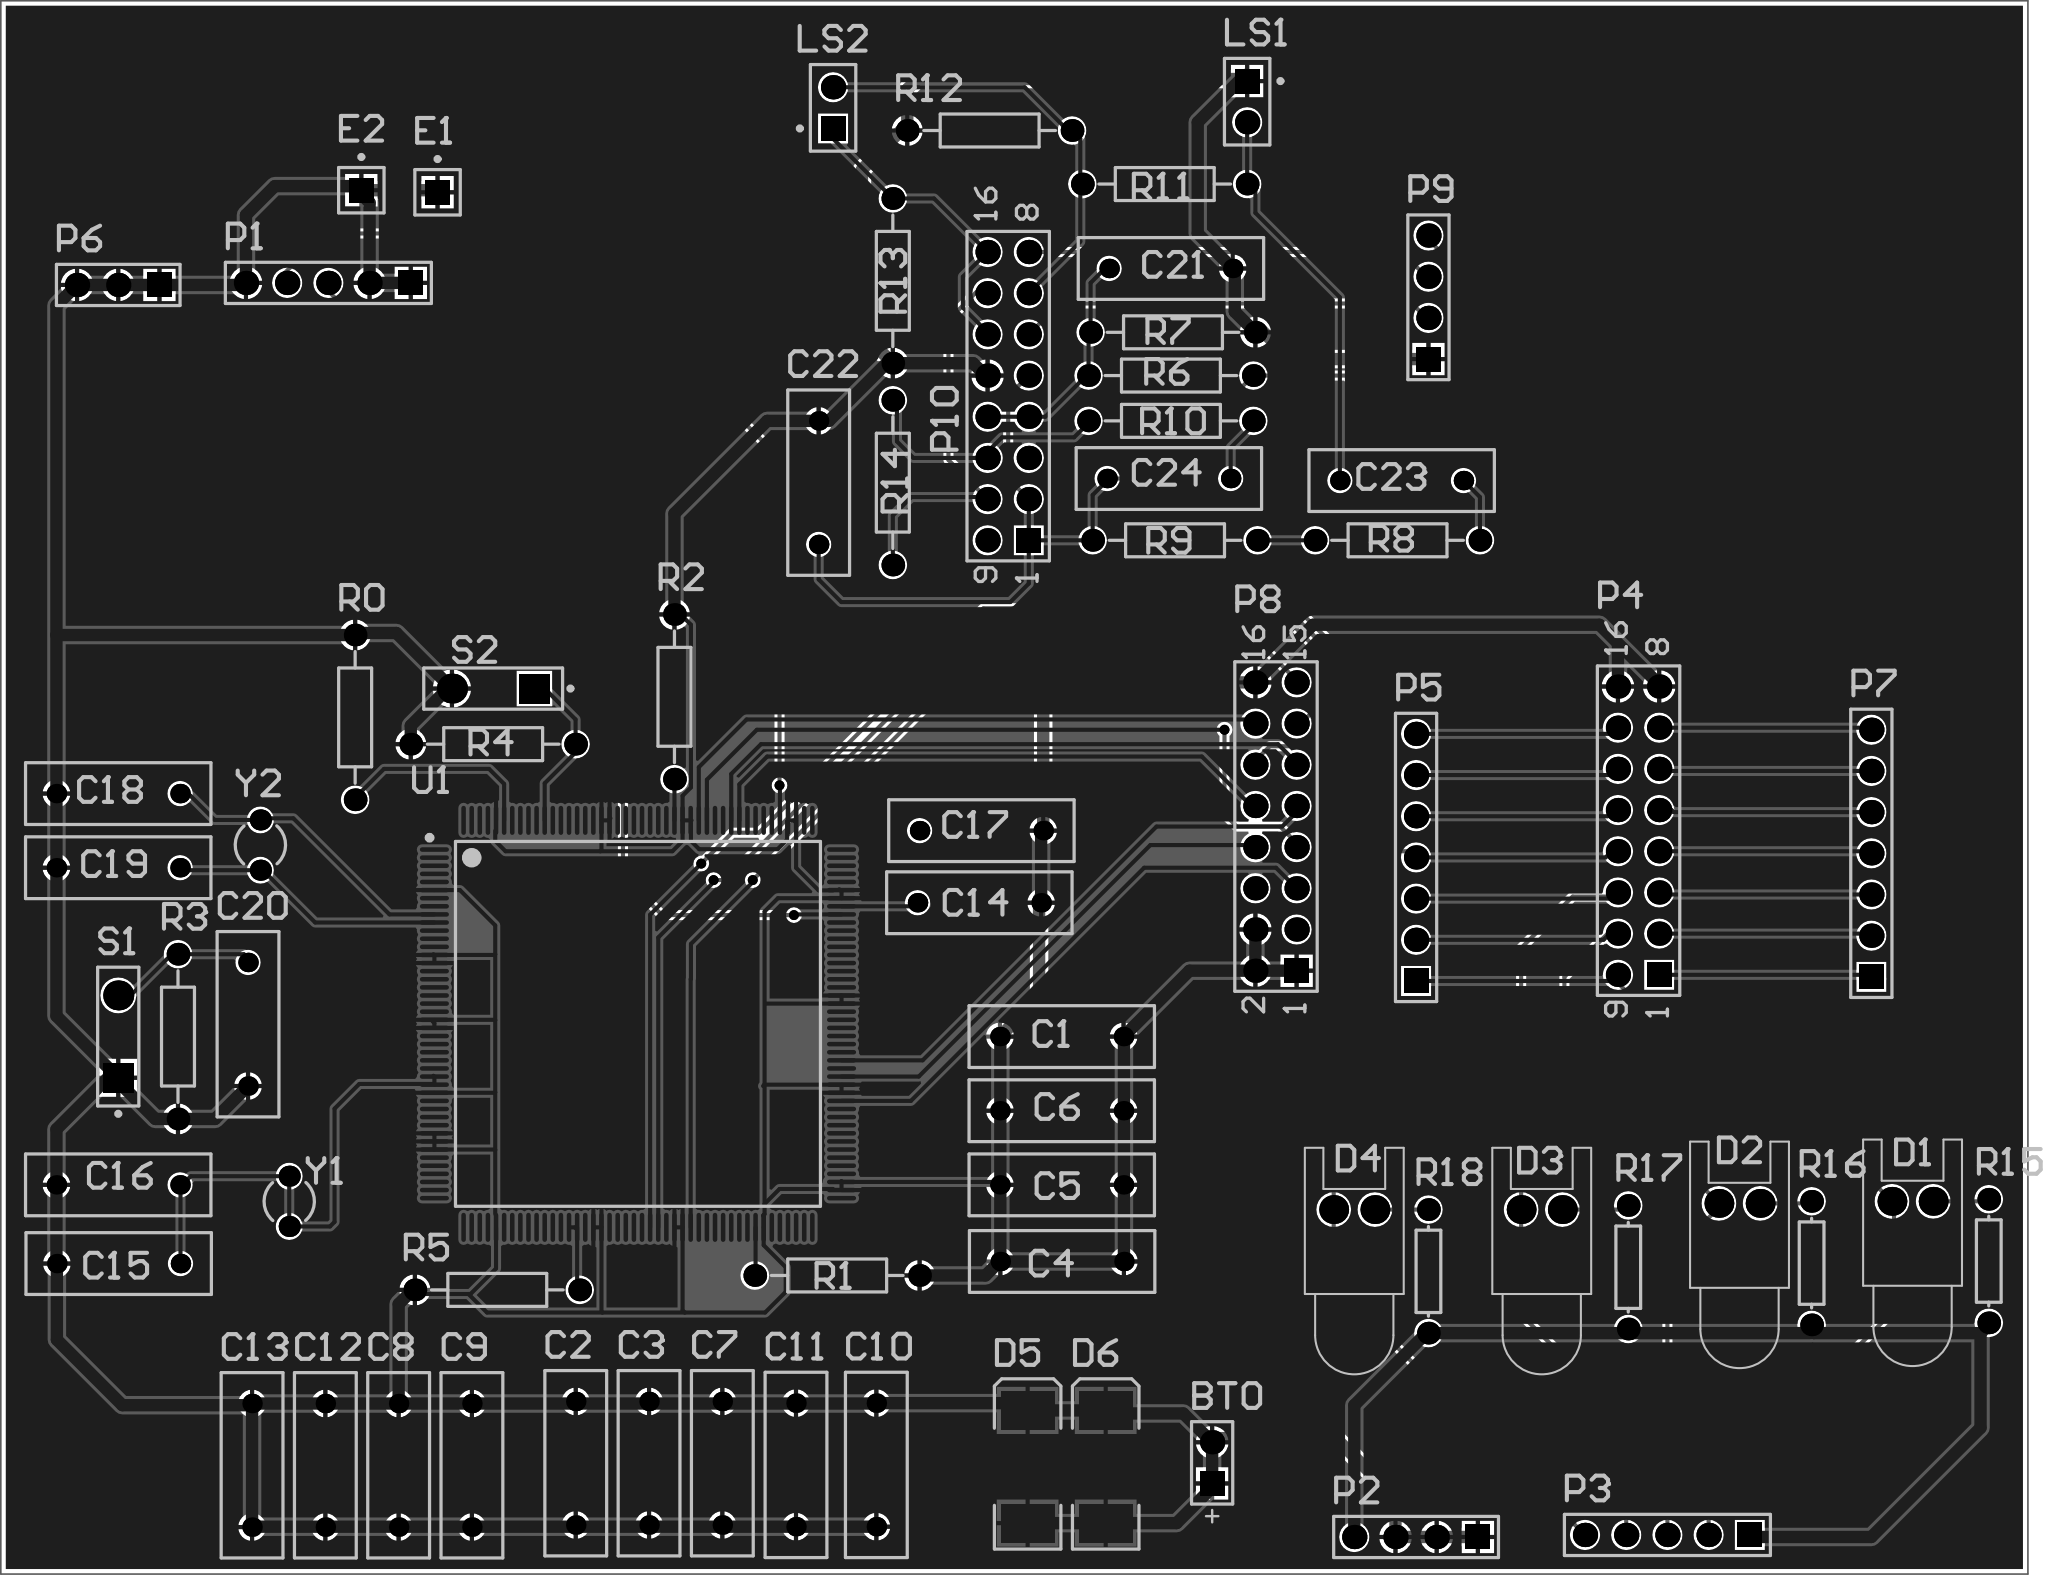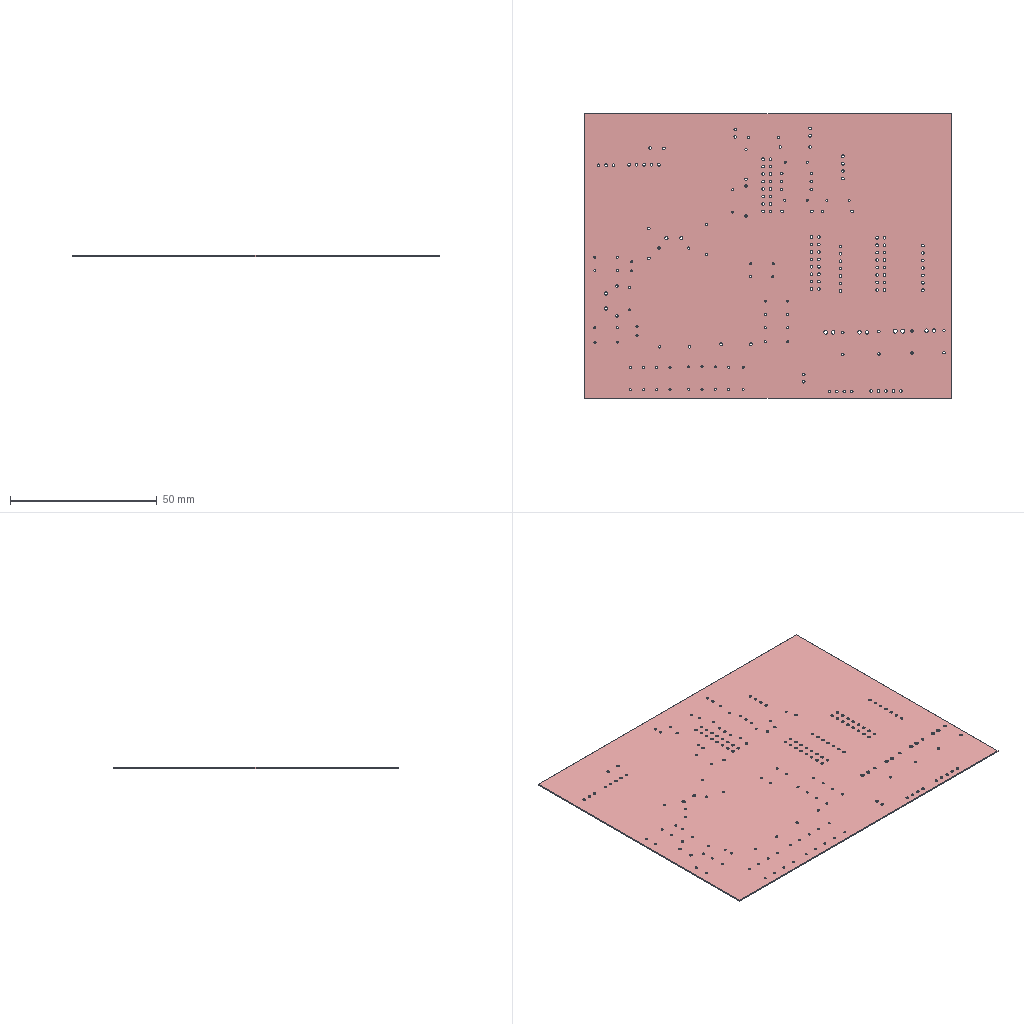Circuit board layout | Altium Designer | box 125 x 97 x 0.4 mm
Layer stack:
# Altium Designer layer stack of  (unit mm; dielectric type: 0 none, 1 core, 2 prepreg, 3 surface material)
index,name,kind,layer,copper_thickness_mm,dielectric_type,dielectric_thickness_mm,dielectric_material,dielectric_constant
0,Top Paste,other,,,,,,
1,Top Overlay,other,,,,,,
2,Top Solder,dielectric,,,3,0.0102,Solder Resist,3.5
3,Top Layer,copper,Top Layer,0.0356,,,,
4,Dielectric1,dielectric,,,0,0.32,FR-4,4.8
5,Bottom Layer,copper,Bottom Layer,0.0356,,,,
6,Bottom Solder,dielectric,,,3,0.0102,Solder Resist,3.5
7,Bottom Overlay,other,,,,,,
8,Bottom Paste,other,,,,,,
# drill layer pairs: low layer,high layer
drill_pair,Top Layer,Bottom Layer
Part placement:
Designator,Comment,Layer,Footprint,Center-X(mm),Center-Y(mm),Rotation
BT0,Battery,TopLayer,BAT-2,125.222,26.035,90
C1,Cap,TopLayer,RAD-0.3,115.951,52.324,180
C2,Cap,TopLayer,RAD-0.3,85.99,26.012,90
C3,Cap,TopLayer,RAD-0.3,90.508,26.012,90
C4,Cap,TopLayer,RAD-0.3,115.975,38.454,180
C5,Cap,TopLayer,RAD-0.3,115.951,43.18,180
C6,Cap,TopLayer,RAD-0.3,115.951,47.752,180
C7,Cap,TopLayer,RAD-0.3,95.026,26.012,90
C8,Cap,TopLayer,RAD-0.3,75.071,25.884,90
C9,Cap,TopLayer,RAD-0.3,79.589,25.884,90
C10,Cap,TopLayer,RAD-0.3,104.521,25.908,90
C11,Cap,TopLayer,RAD-0.3,99.568,25.908,90
C12,Cap,TopLayer,RAD-0.3,70.553,25.884,90
C13,Cap,TopLayer,RAD-0.3,66.035,25.884,90
C14,Cap,TopLayer,RAD-0.3,110.871,60.579,180
C15,Cap,TopLayer,RAD-0.3,57.812,38.326,360
C16,Cap,TopLayer,RAD-0.3,57.785,43.18,360
C17,Cap,TopLayer,RAD-0.3,110.998,65.024,180
C18,Cap,TopLayer,RAD-0.3,57.785,67.31,360
C19,Cap,TopLayer,RAD-0.3,57.785,62.738,360
C20,Cap,TopLayer,RAD-0.3,65.786,53.086,90
C21,Cap,TopLayer,RAD-0.3,122.682,99.695,180
C22,Cap,TopLayer,RAD-0.3,100.965,86.487,270
C23,Cap,TopLayer,RAD-0.3,136.906,86.614,360
C24,Cap,TopLayer,RAD-0.3,122.555,86.741,180
D1,LED1,TopLayer,LED-0,168.402,42.164,360
D2,LED2,TopLayer,LED-0,157.734,42.037,0
D3,LED3,TopLayer,LED-0,145.542,41.656,0
D4,LED4,TopLayer,LED-0,133.985,41.656,0
D5,Diode,TopLayer,DSO-C2/X3.3,113.848,25.794,90
D6,Diode,TopLayer,DSO-C2/X3.3,118.661,25.794,90
E1,Antenna,TopLayer,PIN1,77.47,104.394,0
E2,Antenna,TopLayer,PIN1,72.771,104.521,0
LS1,Bell,TopLayer,PIN2,127.381,109.982,270
LS2,Bell,TopLayer,PIN2,101.854,109.601,90
P1,Header 5,TopLayer,HDR1X5,70.739,98.806,180
P2,Header 4,TopLayer,HDR1X4,137.795,21.463,180
P3,Header 5,TopLayer,HDR1X5,153.289,21.59,180
P4,ULN2003,TopLayer,HDR2X8_CEN,151.511,65.024,90
P5,Header 7,TopLayer,HDR1X7,137.795,63.373,90
P6,Header 3,TopLayer,HDR1X3,57.785,98.679,180
P7,Header 7,TopLayer,HDR1X7,165.862,63.627,90
P8,Header 8X2,TopLayer,HDR2X8,129.159,65.278,90
P9,CON4,TopLayer,HDR1X4,138.557,97.917,90
P10,Header 8X2A,TopLayer,HDR2X8_CEN,112.649,91.821,90
R0,Res2,TopLayer,AXIAL-0.4,72.39,72.009,90
R1,Res2,TopLayer,AXIAL-0.4,102.108,37.592,360
R2,Res2,TopLayer,AXIAL-0.4,92.075,73.279,90
R3,Res2,TopLayer,AXIAL-0.4,61.468,52.324,270
R4,Res2,TopLayer,AXIAL-0.4,80.899,70.358,360
R5,Res2,TopLayer,AXIAL-0.4,81.153,36.703,360
R6,Res2,TopLayer,AXIAL-0.4,122.682,93.091,180
R7,Res2,TopLayer,AXIAL-0.4,122.809,95.758,180
R8,Res2,TopLayer,AXIAL-0.4,136.652,82.931,360
R9,Res2,TopLayer,AXIAL-0.4,122.936,82.931,360
R10,Res2,TopLayer,AXIAL-0.4,122.682,90.297,360
R11,Res2,TopLayer,AXIAL-0.4,122.301,104.902,360
R12,Res2,TopLayer,AXIAL-0.4,111.506,108.204,360
R13,Res2,TopLayer,AXIAL-0.4,105.537,98.933,90
R14,Res2,TopLayer,AXIAL-0.4,105.537,86.487,90
R15,Res1,TopLayer,AXIAL-0.3,173.101,38.481,270
R16,Res1,TopLayer,AXIAL-0.3,162.179,38.354,270
R17,Res1,TopLayer,AXIAL-0.3,150.876,38.1,270
R18,Res1,TopLayer,AXIAL-0.3,138.557,37.846,270
S1,SW-PB,TopLayer,SPST-2,57.785,52.324,90
S2,SW-PB,TopLayer,SPST-2,80.899,73.787,180
U1,Component_1,TopLayer,PCBComponent_1,89.825,53.109,270
Y1,XTAL,TopLayer,BCY-W2/D3.1,68.326,42.164,0
Y2,XTAL,TopLayer,BCY-W2/D3.1,66.548,64.135,180
Pad and via stacks:
# Altium Designer via and pad stacks of  (unit mm). Each distinct definition once, with the count of objects using it.
# via: kind,start_layer,end_layer,hole_mm,diameter_mm,mode(0 simple;1 top-mid-bottom;2 full stack),diameter_per_layer,count,example_net
# pad: kind,layer,hole_mm,hole_type(0 round;1 square;2 slot),plating,top_size,top_shape(1 round;2 rect;3 octagon;9 rounded rect),mid_size,bottom_size,mode,footprint,size_per_layer,count,example
pad,Multi-Layer,0.9,0,plated,1.5x1.5,2,1.5x1.5,1.5x1.5,0,HDR2X8_CEN,,2,P10.1
pad,Multi-Layer,0.9,0,plated,1.5x1.5,1,1.5x1.5,1.5x1.5,0,HDR2X8_CEN,,30,P10.2
pad,Multi-Layer,0.85,0,plated,1.4x1.4,1,1.4x1.4,1.4x1.4,0,AXIAL-0.4,,30,R13.2
pad,Multi-Layer,0.7,0,plated,1.2x1.2,1,1.2x1.2,1.2x1.2,0,RAD-0.3,,48,C21.1
pad,Multi-Layer,1.27,0,plated,1.778x1.778,1,1.778x1.778,1.778x1.778,0,LED-0,,8,D4.2
pad,Multi-Layer,0.7,0,plated,1.3x1.3,1,1.3x1.3,1.3x1.3,0,BCY-W2/D3.1,,4,Y1.1
pad,Multi-Layer,1.1,0,plated,1.85x1.85,1,1.85x1.85,1.85x1.85,0,SPST-2,,2,S2.2
pad,Multi-Layer,1.1,0,plated,1.85x1.85,2,1.85x1.85,1.85x1.85,0,SPST-2,,2,S2.1
pad,Multi-Layer,0.9,0,plated,1.5x1.5,1,1.5x1.5,1.5x1.5,0,PIN2,,2,LS2.2
pad,Multi-Layer,0.9,0,plated,1.5x1.5,2,1.5x1.5,1.5x1.5,0,PIN2,,2,LS2.1
pad,Multi-Layer,0.9,0,plated,1.5x1.5,2,1.5x1.5,1.5x1.5,0,BAT-2,,1,BT0.1
pad,Multi-Layer,0.9,0,plated,1.5x1.5,1,1.5x1.5,1.5x1.5,0,BAT-2,,1,BT0.2
pad,Multi-Layer,0.9,0,plated,1.5x1.5,2,1.5x1.5,1.5x1.5,0,HDR1X4,,2,P9.1
pad,Multi-Layer,0.9,0,plated,1.5x1.5,1,1.5x1.5,1.5x1.5,0,HDR1X4,,6,P9.2
pad,Multi-Layer,0.9,0,plated,1.5x1.5,2,1.5x1.5,1.5x1.5,0,HDR1X5,,2,P1.1
pad,Multi-Layer,0.9,0,plated,1.5x1.5,1,1.5x1.5,1.5x1.5,0,HDR1X5,,8,P1.2
pad,Multi-Layer,0.9,0,plated,1.5x1.5,1,1.5x1.5,1.5x1.5,0,HDR2X8,,15,P8.16
pad,Multi-Layer,0.9,0,plated,1.5x1.5,2,1.5x1.5,1.5x1.5,0,HDR2X8,,1,P8.1
pad,Multi-Layer,0.9,0,plated,1.5x1.5,2,1.5x1.5,1.5x1.5,0,PIN1,,2,E1.1
pad,Multi-Layer,0.9,0,plated,1.5x1.5,1,1.5x1.5,1.5x1.5,0,HDR1X3,,2,P6.3
pad,Multi-Layer,0.9,0,plated,1.5x1.5,2,1.5x1.5,1.5x1.5,0,HDR1X3,,1,P6.1
pad,Multi-Layer,0.9,0,plated,1.5x1.5,1,1.5x1.5,1.5x1.5,0,HDR1X7,,12,P5.3
pad,Multi-Layer,0.9,0,plated,1.5x1.5,2,1.5x1.5,1.5x1.5,0,HDR1X7,,2,P5.1
pad,Multi-Layer,0.85,0,plated,1.4x1.4,1,1.4x1.4,1.4x1.4,0,AXIAL-0.3,,8,R15.1
pad,Top Layer,0,0,plated,2.4x3.3,2,2.4x3.3,2.4x3.3,0,DSO-C2/X3.3,,4,D6.2
pad,Top Layer,0,0,plated,0.28x1.8,1,0.28x1.8,0.28x1.8,0,PCBComponent_1,,176,U1.176
via,Top Layer,Bottom Layer,0.3048,0.6096,0,,6,PD4/FSMC_NOE
Copper pours:
name,layer,net,type(0 solid;1 hatched;2 none)
D,Bottom Layer,BAT_CR1220,0
D,Top Layer,BAT_CR1220,0
Design rules, without the lines most boards share:
# Altium Designer design rules of  (exported by Altium Designer, unit mm)
# columns: name | kind | enabled | priority | scope1 | scope2 | descriptor | typed fields (field=value)
Clearance | 0 | enabled | 1 | All | All | Clearance Constraint (Gap=7mil) (All),(All) | gap=0.1778
PlaneConnect | 6 | enabled | 1 | All | All | Power Plane Connect Rule(Relief Connect )(Expansion=20mil) (Conductor Width=10mil) (Air Gap=10mil) (Entries=4) (All) | relief_conductor_width=0.254 relief_entries=4 relief_expansion=0.508
PolygonConnect | 20 | enabled | 1 | All | All | Polygon Connect Rule(Relief Connect )(Conductor Width=10mil) (Relief Angle=90 Angle) (Entries=4) (Air Gap Width=10mil) (All),(All) | connect_style(0=relief,1=direct,2=none)=0 relief_conductor_width=0.254 relief_entries=4
Width | 2 | enabled | 1 | All | All | Width Constraint (Min=10mil) (Max=30mil) (Preferred=10mil) (All) |
RoutingVias | 11 | enabled | 1 | All | All | Routing Via (MinHoleWidth=28mil) (MaxHoleWidth=28mil) (PreferredHoleWidth=28mil) (MinWidth=50mil) (MaxWidth=50mil) (PreferedWidth=50mil) (All) | via_min_hole=0.7112 via_max_hole=0.7112 via_preferred_diameter=1.27 via_preferred_hole=0.7112
PasteMaskExpansion | 14 | enabled | 1 | All | All | Paste Mask Expansion (Expansion =0mil) (All) | expansion=0
SolderMaskExpansion | 13 | enabled | 1 | All | All | Solder Mask Expansion (Expansion =4mil) (All) | expansion=0.1016
DiffPairsRouting | 51 | enabled | 1 | All | All | Differential Pairs Uncoupled Length using the Gap Constraints (Min=10mil) (Max=10mil) (Prefered=10mil)  and Width Constraints (Min=15mil) (Max=15mil) (Prefered=15mil) (All) |
HoleToHoleClearance | 52 | enabled | 1 | All | All | Hole To Hole Clearance (Gap=10mil) (All),(All) | gap=0.254
MinimumSolderMaskSliver | 53 | enabled | 1 | All | All | Minimum Solder Mask Sliver (Gap=0mil) (All),(All) |
SilkscreenOverComponentPads | 54 | enabled | 1 | IsPad | All | Silk To Solder Mask (Clearance=0mil) (IsPad),(All) |
SilkToSilkClearance | 55 | enabled | 1 | All | All | Silk to Silk (Clearance=0mil) (All),(All) |